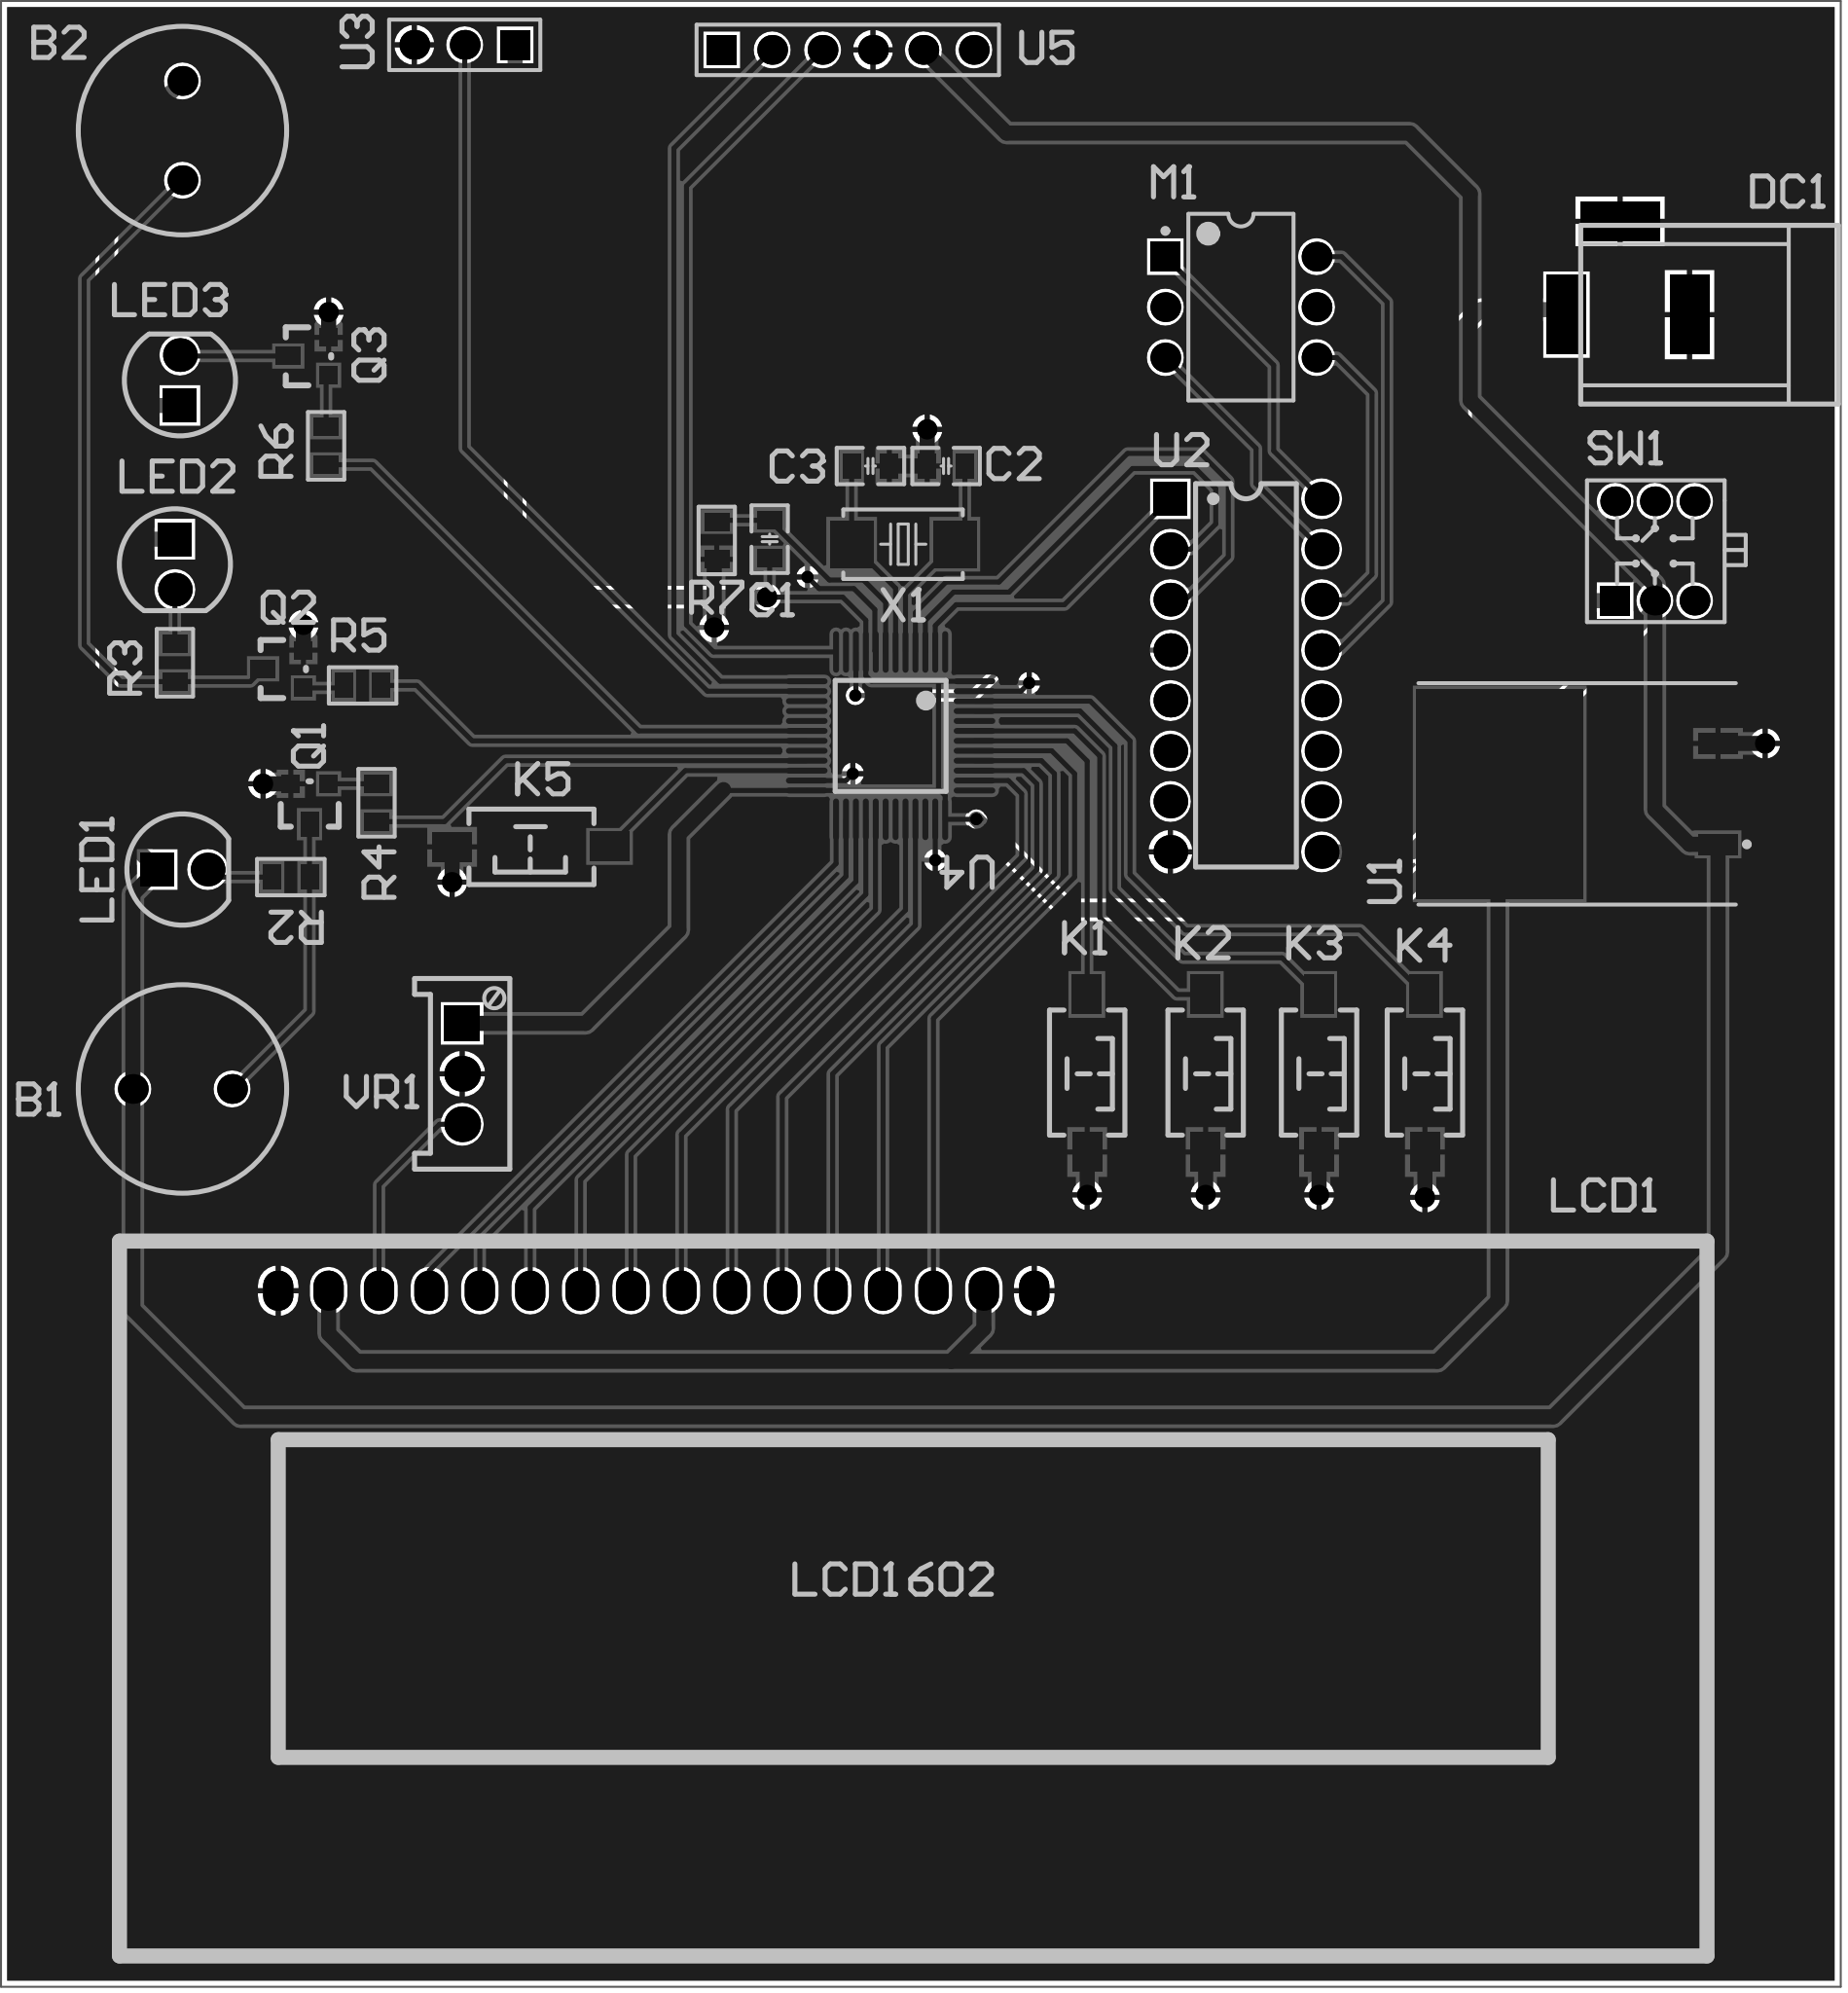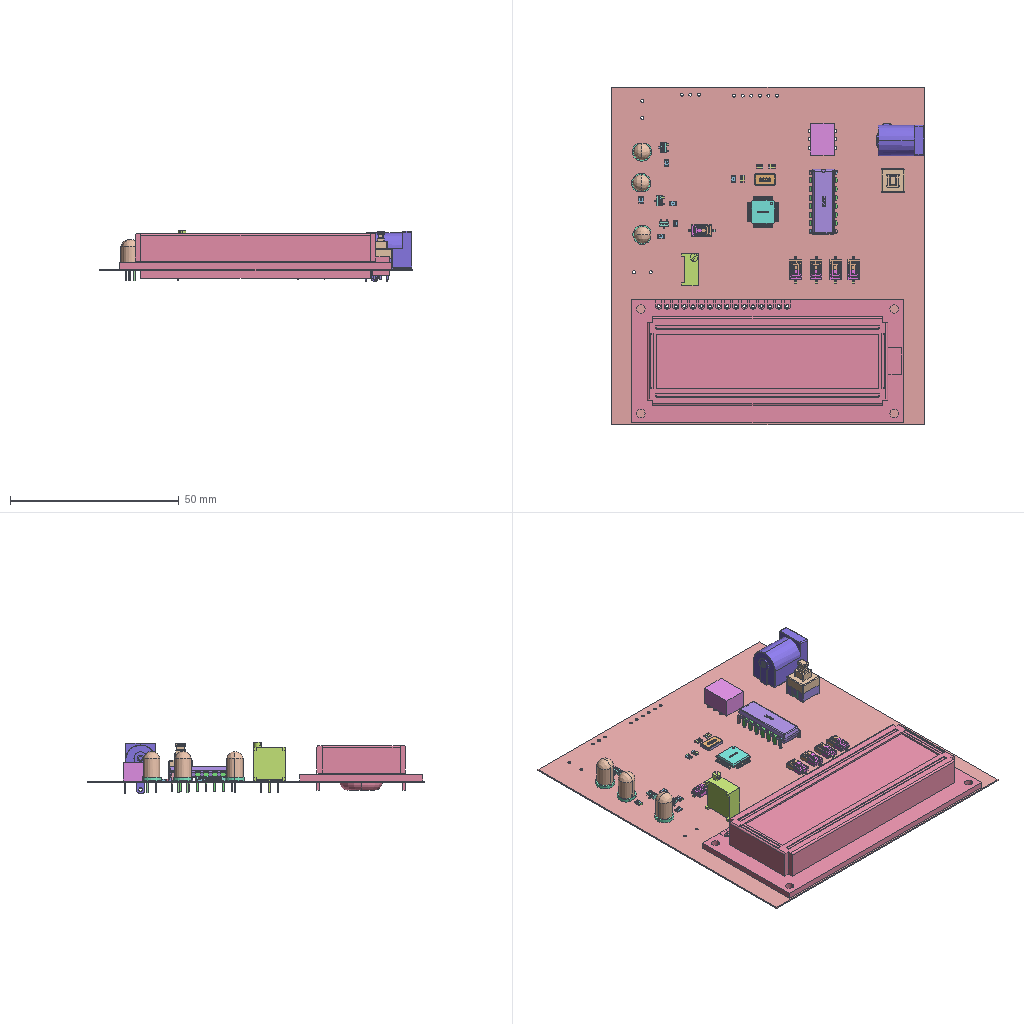Circuit board layout | Altium Designer | box 92.7 x 100 x 15.3 mm
Layer stack:
# Altium Designer layer stack of  (unit mm; dielectric type: 0 none, 1 core, 2 prepreg, 3 surface material)
index,name,kind,layer,copper_thickness_mm,dielectric_type,dielectric_thickness_mm,dielectric_material,dielectric_constant
0,Top Paste,other,,,,,,
1,Top Overlay,other,,,,,,
2,Top Solder,dielectric,,,3,0.0102,Solder Resist,3.5
3,Top Layer,copper,Top Layer,0.0356,,,,
4,Dielectric 1,dielectric,,,0,0.32,FR-4,4.8
5,Bottom Layer,copper,Bottom Layer,0.0356,,,,
6,Bottom Solder,dielectric,,,3,0.0102,Solder Resist,3.5
7,Bottom Overlay,other,,,,,,
8,Bottom Paste,other,,,,,,
# drill layer pairs: low layer,high layer
drill_pair,Top Layer,Bottom Layer
Part placement:
Designator,Comment,Layer,Footprint,Center-X(mm),Center-Y(mm),Rotation
Q1,8050,TopLayer,SOT-23,40.958,84.963,180
X1,8MHz,TopLayer,OSC_6035-2P,70.866,98.044,180
VR1,50K,TopLayer,3296W,48.641,71.374,270
U5,HC05 Bluetooth module,TopLayer,HDR1X6,68.072,122.936,360
U4,STM32F103C,TopLayer,LQFP48_7X7,70.231,88.405,180
U3,DHT11,TopLayer,HDR1X3,48.768,123.19,180
U2,ULN2003,TopLayer,DIP16,88.138,91.44,360
U1,LM1117-3.3V,TopLayer,D2PAK,106.426,85.471,90
SW1,SW-DPDT,TopLayer,KFT_DIP-7X7,108.744,97.703,0
R7,10K,TopLayer,R_0805_L,61.468,98.232,270
R6,10K,TopLayer,R_0805_L,41.783,102.997,90
R5,10K,TopLayer,R_0805_L,43.622,90.932,180
R4,10K,TopLayer,R_0805_L,44.323,85.024,90
R3,510R,TopLayer,R_0805_L,34.163,92.075,90
R2,510R,TopLayer,R_0805_L,40.005,81.28,180
Q3,8050,TopLayer,SOT-23,40.894,107.505,90
Q2,8050,TopLayer,SOT-23,39.624,91.757,90
M1,STEP,TopLayer,DIP-6,87.884,109.982,0
LED3,LED,TopLayer,LED_5MM-W,34.417,106.299,90
LED2,LED_G,TopLayer,LED_5MM-W,34.163,97.028,270
LED1,LED_G,TopLayer,LED_5MM-W,34.544,81.661,360
LCD1,LCD1602,TopLayer,LCD1602,58.42,60.452,360
K5,SW-BUTTON,TopLayer,TSW_SMD-3*6*2.5,52.099,82.814,180
K4,SW-BUTTON,TopLayer,TSW_SMD-3*6*2.5,97.145,71.403,270
K3,SW-BUTTON,TopLayer,TSW_SMD-3*6*2.5,91.811,71.403,270
K2,SW-BUTTON,TopLayer,TSW_SMD-3*6*2.5,86.096,71.403,270
K1,SW-BUTTON,TopLayer,TSW_SMD-3*6*2.5,80.127,71.403,270
DC1,DC005-2.5MM,TopLayer,DC-005,107.39,111.951,360
C3,20pF,TopLayer,C_0805_L,69.215,101.981,0
C2,20pF,TopLayer,C_0805_L,73.025,101.981,180
C1,1uF,TopLayer,C_0805_L,64.135,98.298,90
B2,Heater plate,TopLayer,RB5-10.5,34.544,118.872,270
B1,Fan,TopLayer,RB5-10.5,34.544,70.612,360
Pad and via stacks:
# Altium Designer via and pad stacks of  (unit mm). Each distinct definition once, with the count of objects using it.
# via: kind,start_layer,end_layer,hole_mm,diameter_mm,mode(0 simple;1 top-mid-bottom;2 full stack),diameter_per_layer,count,example_net
# pad: kind,layer,hole_mm,hole_type(0 round;1 square;2 slot),plating,top_size,top_shape(1 round;2 rect;3 octagon;9 rounded rect),mid_size,bottom_size,mode,footprint,size_per_layer,count,example
pad,Multi-Layer,0.9,0,plated,1.524x2.032,1,1.524x2.032,1.524x2.032,0,LCD1602,,16,LCD1.1
pad,Multi-Layer,0.9,0,plated,1.5x1.5,1,1.5x1.5,1.5x1.5,0,DIP-6,,5,M1.4
pad,Multi-Layer,0.9,0,plated,1.5x1.5,2,1.5x1.5,1.5x1.5,0,DIP-6,,1,M1.1
pad,Multi-Layer,0.9,0,plated,1.5x1.5,1,1.5x1.5,1.5x1.5,0,KFT DIP-7X7,,5,SW1.4
pad,Multi-Layer,0.9,0,plated,1.5x1.5,2,1.5x1.5,1.5x1.5,0,KFT DIP-7X7,,1,SW1.1
pad,Multi-Layer,0.8,2,plated,2x4,2,2x4,2x4,0,DC-005,,2,DC1.1
pad,Multi-Layer,0.8,2,plated,4x2,2,4x2,4x2,0,DC-005,,1,DC1.3
pad,Multi-Layer,0.8,0,plated,1.7x1.7,1,1.7x1.7,1.7x1.7,0,DIP16,,15,U2.16
pad,Multi-Layer,0.8,0,plated,1.7x1.7,2,1.7x1.7,1.7x1.7,0,DIP16,,1,U2.1
pad,Multi-Layer,0.9,0,plated,1.5x1.5,2,1.5x1.5,1.5x1.5,0,HDR1X3,,1,U3.1
pad,Multi-Layer,0.9,0,plated,1.5x1.5,1,1.5x1.5,1.5x1.5,0,HDR1X3,,2,U3.2
pad,Multi-Layer,0.7,0,plated,1.8x1.8,1,1.8x1.8,1.8x1.8,0,3296W,,2,VR1.3
pad,Multi-Layer,0.7,0,plated,1.8x1.8,2,1.8x1.8,1.8x1.8,0,3296W,,1,VR1.1
pad,Multi-Layer,0.9,0,plated,1.7x1.7,1,1.7x1.7,1.7x1.7,0,LED 5MM-W,,3,LED2.2
pad,Multi-Layer,0.9,0,plated,1.7x1.7,2,1.7x1.7,1.7x1.7,0,LED 5MM-W,,3,LED2.1
pad,Multi-Layer,0.9,0,plated,1.5x1.5,1,1.5x1.5,1.5x1.5,0,RB5-10.5,,4,B2.1
pad,Multi-Layer,0.9,0,plated,1.5x1.5,2,1.5x1.5,1.5x1.5,0,HDR1X6,,1,U5.1
pad,Multi-Layer,0.9,0,plated,1.5x1.5,1,1.5x1.5,1.5x1.5,0,HDR1X6,,5,U5.2
pad,Top Layer,0,0,plated,0.9144x0.9144,2,0.9144x0.9144,0.9144x0.9144,0,SOT-23,,6,Q1.B
pad,Top Layer,0,0,plated,0.9144x1.27,2,0.9144x1.27,0.9144x1.27,0,SOT-23,,3,Q1.C
pad,Top Layer,0,0,plated,1.05x2,2,1.05x2,1.05x2,0,D2PAK,,2,U1.3
pad,Top Layer,0,0,plated,10.55x8.4,2,10.55x8.4,10.55x8.4,0,D2PAK,,1,U1.2
pad,Top Layer,0,0,plated,0.3x2.1,1,0.3x2.1,0.3x2.1,0,LQFP48 7X7,,48,U4.48
pad,Top Layer,0,0,plated,1.27x0.889,2,1.27x0.889,1.27x0.889,0,R 0805_L,,12,R3.1
pad,Top Layer,0,0,plated,1.27x0.889,2,1.27x0.889,1.27x0.889,0,C 0805_L,,6,C1.1
pad,Top Layer,0,0,unplated,2.4x2.2,2,2.4x2.2,2.4x2.2,0,OSC 6035-2P,,2,X1.1
pad,Top Layer,0,0,plated,2x1.5,2,2x1.5,2x1.5,0,TSW SMD-3*6*2.5,,10,K5.1
via,Top Layer,Bottom Layer,0.3048,0.6096,0,,6,GND
via,Top Layer,Bottom Layer,0.635,1.016,0,,13,GND
Copper pours:
name,layer,net,type(0 solid;1 hatched;2 none)
D,Top Layer,GND,0
D,Bottom Layer,GND,0
Design rules, without the lines most boards share:
# Altium Designer design rules of  (exported by Altium Designer, unit mm)
# columns: name | kind | enabled | priority | scope1 | scope2 | descriptor | typed fields (field=value)
SilkToSilkClearance | 55 | enabled | 1 | All | All | Silk to Silk (Clearance=0mil) (All),(All) |
SilkToSolderMaskClearance | 54 | enabled | 1 | IsPad | All | Silk To Solder Mask (Clearance=0mil) (IsPad),(All) |
MinimumSolderMaskSliver | 53 | enabled | 1 | All | All | Minimum Solder Mask Sliver (Gap=0mil) (All),(All) |
HoleToHoleClearance | 52 | enabled | 1 | All | All | Hole To Hole Clearance (Gap=10mil) (All),(All) | gap=0.254
DiffPairsRouting | 51 | enabled | 1 | All | All | Differential Pairs Uncoupled Length using the Gap Constraints (Min=10mil) (Max=10mil) (Prefered=10mil)  and Width Constraints (Min=15mil) (Max=15mil) (Prefered=15mil) (All) |
HoleSize | 42 | enabled | 1 | All | All | Hole Size Constraint (Min=1mil) (Max=11111mil) (All) |
SolderMaskExpansion | 13 | enabled | 1 | All | All | Solder Mask Expansion (Expansion =4mil) (All) | expansion=0.1016
PasteMaskExpansion | 14 | enabled | 1 | All | All | Paste Mask Expansion (Expansion =0mil) (All) | expansion=0
RoutingVias | 11 | enabled | 1 | All | All | Routing Via (MinHoleWidth=28mil) (MaxHoleWidth=28mil) (PreferredHoleWidth=28mil) (MinWidth=50mil) (MaxWidth=50mil) (PreferedWidth=50mil) (All) | via_min_hole=0.7112 via_max_hole=0.7112 via_preferred_diameter=1.27 via_preferred_hole=0.7112
Width | 2 | enabled | 1 | All | All | Width Constraint (Min=10mil) (Max=888mil) (Preferred=10mil) (All) |
PolygonConnect | 20 | enabled | 1 | All | All | Polygon Connect Rule(Relief Connect )(Conductor Width=10mil) (Relief Angle=90 Angle) (Entries=4) (Air Gap Width=10mil) (All),(All) | connect_style(0=relief,1=direct,2=none)=0 relief_conductor_width=0.254 relief_entries=4
PlaneConnect | 6 | enabled | 1 | All | All | Power Plane Connect Rule(Relief Connect )(Expansion=20mil) (Conductor Width=10mil) (Air Gap=10mil) (Entries=4) (All) | relief_conductor_width=0.254 relief_entries=4 relief_expansion=0.508
Clearance | 0 | enabled | 1 | All | All | Clearance Constraint (Gap=7mil) (All),(All) | gap=0.1778
Classes set for this board:
# Altium Designer classes of  (member kind: 0 net, 1 component, 2 from-to, 3 pad, 4 layer, 5 differential pair, 6 design channel, 7 polygon, 8 structure, 9 xSignal)
# columns: class name | member kind | superclass | members
AD | 1 | no | B1; B2; C1; C2; C3; DC1; K1; K2; K3; K4; K5; LCD1; LED1; LED2; LED3; M1; Q2; Q3; R2; R3; R4; R5; R6; R7; SW1; U1; U2; U3; U4; U5; VR1; X1; Q1;